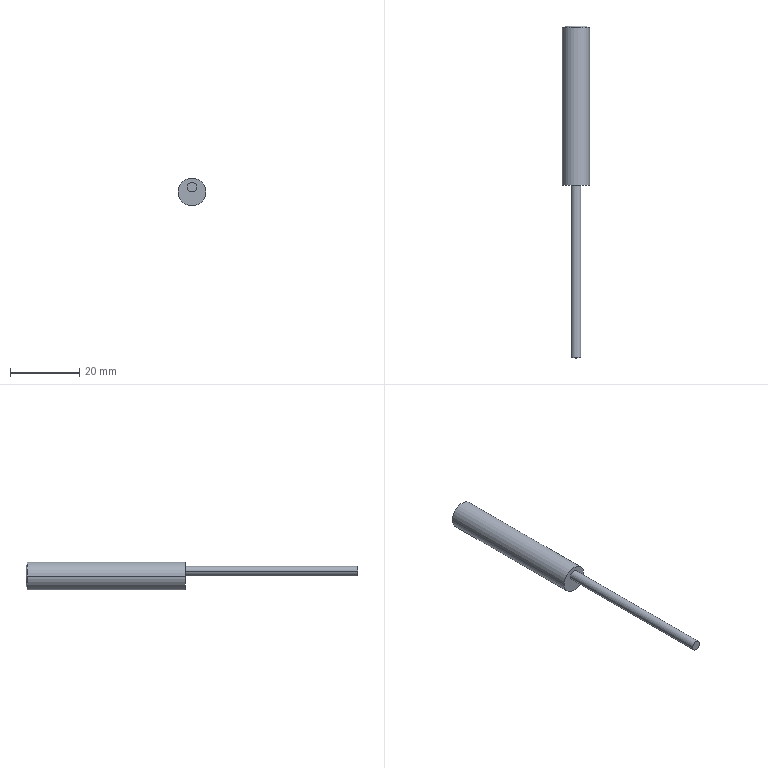Part | SolidWorks | features BaseBody 1, ICE 1, RefSurface 1 | 1 solid | 10 faces | box 8 x 96 x 8 mm | volume 2614 mm3 | cylinder 4 | plane 4 | cone 2 | commonest cylinder face diameters 2.8 x2 8 x2
STEP:
#1=CARTESIAN_POINT('',(-1.4,-46.,1.4));
#2=VERTEX_POINT('',#1);
#3=CARTESIAN_POINT('',(1.4,-46.,1.4));
#4=VERTEX_POINT('',#3);
#5=CARTESIAN_POINT('',(0.,-46.,1.4));
#6=DIRECTION('',(0.,1.,0.));
#7=DIRECTION('',(1.,0.,0.));
#8=AXIS2_PLACEMENT_3D('',#5,#6,#7);
#9=CIRCLE('',#8,1.4);
#10=EDGE_CURVE('',#2,#4,#9,.T.);
#11=ORIENTED_EDGE('',*,*,#10,.F.);
#12=CARTESIAN_POINT('',(-1.4,-96.,1.4));
#13=VERTEX_POINT('',#12);
#14=CARTESIAN_POINT('',(-1.4,-46.,1.4));
#15=DIRECTION('',(0.,-1.,0.));
#16=VECTOR('',#15,1000.);
#17=LINE('',#14,#16);
#18=EDGE_CURVE('',#2,#13,#17,.T.);
#19=ORIENTED_EDGE('',*,*,#18,.T.);
#20=CARTESIAN_POINT('',(1.4,-96.,1.4));
#21=VERTEX_POINT('',#20);
#22=CARTESIAN_POINT('',(0.,-96.,1.4));
#23=DIRECTION('',(0.,1.,0.));
#24=DIRECTION('',(1.,0.,0.));
#25=AXIS2_PLACEMENT_3D('',#22,#23,#24);
#26=CIRCLE('',#25,1.4);
#27=EDGE_CURVE('',#13,#21,#26,.T.);
#28=ORIENTED_EDGE('',*,*,#27,.T.);
#29=CARTESIAN_POINT('',(1.4,-46.,1.4));
#30=DIRECTION('',(0.,-1.,0.));
#31=VECTOR('',#30,1000.);
#32=LINE('',#29,#31);
#33=EDGE_CURVE('',#4,#21,#32,.T.);
#34=ORIENTED_EDGE('',*,*,#33,.F.);
#35=EDGE_LOOP('',(#11,#19,#28,#34));
#36=FACE_OUTER_BOUND('',#35,.T.);
#37=CARTESIAN_POINT('',(0.,-46.,1.4));
#38=DIRECTION('',(0.,-1.,0.));
#39=DIRECTION('',(1.,0.,0.));
#40=AXIS2_PLACEMENT_3D('',#37,#38,#39);
#41=CYLINDRICAL_SURFACE('',#40,1.4);
#42=ADVANCED_FACE('',(#36),#41,.T.);
#43=CARTESIAN_POINT('',(3.,0.,0.));
#44=VERTEX_POINT('',#43);
#45=CARTESIAN_POINT('',(-3.,0.,0.));
#46=VERTEX_POINT('',#45);
#47=CARTESIAN_POINT('',(0.,0.,0.));
#48=DIRECTION('',(0.,-1.,0.));
#49=DIRECTION('',(1.,0.,0.));
#50=AXIS2_PLACEMENT_3D('',#47,#48,#49);
#51=CIRCLE('',#50,3.);
#52=EDGE_CURVE('',#44,#46,#51,.T.);
#53=ORIENTED_EDGE('',*,*,#52,.T.);
#54=CARTESIAN_POINT('',(-3.3,-0.3,0.));
#55=VERTEX_POINT('',#54);
#56=CARTESIAN_POINT('',(-3.3,-0.3,0.));
#57=DIRECTION('',(-0.7071,-0.7071,0.));
#58=VECTOR('',#57,1000.);
#59=LINE('',#56,#58);
#60=EDGE_CURVE('',#46,#55,#59,.T.);
#61=ORIENTED_EDGE('',*,*,#60,.T.);
#62=CARTESIAN_POINT('',(3.3,-0.3,0.));
#63=VERTEX_POINT('',#62);
#64=CARTESIAN_POINT('',(0.,-0.3,0.));
#65=DIRECTION('',(0.,-1.,0.));
#66=DIRECTION('',(1.,0.,0.));
#67=AXIS2_PLACEMENT_3D('',#64,#65,#66);
#68=CIRCLE('',#67,3.3);
#69=EDGE_CURVE('',#63,#55,#68,.T.);
#70=ORIENTED_EDGE('',*,*,#69,.F.);
#71=CARTESIAN_POINT('',(3.3,-0.3,0.));
#72=DIRECTION('',(0.7071,-0.7071,0.));
#73=VECTOR('',#72,1000.);
#74=LINE('',#71,#73);
#75=EDGE_CURVE('',#44,#63,#74,.T.);
#76=ORIENTED_EDGE('',*,*,#75,.F.);
#77=EDGE_LOOP('',(#53,#61,#70,#76));
#78=FACE_OUTER_BOUND('',#77,.T.);
#79=CARTESIAN_POINT('',(0.,-0.3,0.));
#80=DIRECTION('',(0.,-1.,0.));
#81=DIRECTION('',(1.,0.,0.));
#82=AXIS2_PLACEMENT_3D('',#79,#80,#81);
#83=CONICAL_SURFACE('',#82,3.3,0.7854);
#84=ADVANCED_FACE('',(#78),#83,.T.);
#85=CARTESIAN_POINT('',(-4.,-46.,0.));
#86=VERTEX_POINT('',#85);
#87=CARTESIAN_POINT('',(4.,-46.,0.));
#88=VERTEX_POINT('',#87);
#89=CARTESIAN_POINT('',(0.,-46.,0.));
#90=DIRECTION('',(0.,1.,0.));
#91=DIRECTION('',(1.,0.,0.));
#92=AXIS2_PLACEMENT_3D('',#89,#90,#91);
#93=CIRCLE('',#92,4.);
#94=EDGE_CURVE('',#86,#88,#93,.T.);
#95=ORIENTED_EDGE('',*,*,#94,.T.);
#96=CARTESIAN_POINT('',(4.,-0.3,0.));
#97=VERTEX_POINT('',#96);
#98=CARTESIAN_POINT('',(4.,-57.314,0.));
#99=DIRECTION('',(0.,1.,0.));
#100=VECTOR('',#99,1000.);
#101=LINE('',#98,#100);
#102=EDGE_CURVE('',#88,#97,#101,.T.);
#103=ORIENTED_EDGE('',*,*,#102,.T.);
#104=CARTESIAN_POINT('',(-4.,-0.3,0.));
#105=VERTEX_POINT('',#104);
#106=CARTESIAN_POINT('',(0.,-0.3,0.));
#107=DIRECTION('',(0.,1.,0.));
#108=DIRECTION('',(-1.,0.,0.));
#109=AXIS2_PLACEMENT_3D('',#106,#107,#108);
#110=CIRCLE('',#109,4.);
#111=EDGE_CURVE('',#105,#97,#110,.T.);
#112=ORIENTED_EDGE('',*,*,#111,.F.);
#113=CARTESIAN_POINT('',(-4.,-57.314,0.));
#114=DIRECTION('',(0.,1.,0.));
#115=VECTOR('',#114,1000.);
#116=LINE('',#113,#115);
#117=EDGE_CURVE('',#86,#105,#116,.T.);
#118=ORIENTED_EDGE('',*,*,#117,.F.);
#119=EDGE_LOOP('',(#95,#103,#112,#118));
#120=FACE_OUTER_BOUND('',#119,.T.);
#121=CARTESIAN_POINT('',(0.,-57.314,0.));
#122=DIRECTION('',(0.,1.,0.));
#123=DIRECTION('',(-1.,0.,0.));
#124=AXIS2_PLACEMENT_3D('',#121,#122,#123);
#125=CYLINDRICAL_SURFACE('',#124,4.);
#126=ADVANCED_FACE('',(#120),#125,.T.);
#127=ORIENTED_EDGE('',*,*,#102,.F.);
#128=CARTESIAN_POINT('',(0.,-46.,0.));
#129=DIRECTION('',(0.,1.,0.));
#130=DIRECTION('',(1.,0.,0.));
#131=AXIS2_PLACEMENT_3D('',#128,#129,#130);
#132=CIRCLE('',#131,4.);
#133=EDGE_CURVE('',#88,#86,#132,.T.);
#134=ORIENTED_EDGE('',*,*,#133,.T.);
#135=ORIENTED_EDGE('',*,*,#117,.T.);
#136=CARTESIAN_POINT('',(0.,-0.3,0.));
#137=DIRECTION('',(0.,1.,0.));
#138=DIRECTION('',(-1.,0.,0.));
#139=AXIS2_PLACEMENT_3D('',#136,#137,#138);
#140=CIRCLE('',#139,4.);
#141=EDGE_CURVE('',#97,#105,#140,.T.);
#142=ORIENTED_EDGE('',*,*,#141,.F.);
#143=EDGE_LOOP('',(#127,#134,#135,#142));
#144=FACE_OUTER_BOUND('',#143,.T.);
#145=CARTESIAN_POINT('',(0.,-57.314,0.));
#146=DIRECTION('',(0.,1.,0.));
#147=DIRECTION('',(-1.,0.,0.));
#148=AXIS2_PLACEMENT_3D('',#145,#146,#147);
#149=CYLINDRICAL_SURFACE('',#148,4.);
#150=ADVANCED_FACE('',(#144),#149,.T.);
#151=ORIENTED_EDGE('',*,*,#52,.F.);
#152=CARTESIAN_POINT('',(0.,0.,0.));
#153=DIRECTION('',(0.,-1.,0.));
#154=DIRECTION('',(1.,0.,0.));
#155=AXIS2_PLACEMENT_3D('',#152,#153,#154);
#156=CIRCLE('',#155,3.);
#157=EDGE_CURVE('',#46,#44,#156,.T.);
#158=ORIENTED_EDGE('',*,*,#157,.F.);
#159=EDGE_LOOP('',(#151,#158));
#160=FACE_OUTER_BOUND('',#159,.T.);
#161=CARTESIAN_POINT('',(3.3,0.,0.));
#162=DIRECTION('',(0.,1.,0.));
#163=DIRECTION('',(-1.,0.,0.));
#164=AXIS2_PLACEMENT_3D('',#161,#162,#163);
#165=PLANE('',#164);
#166=ADVANCED_FACE('',(#160),#165,.T.);
#167=ORIENTED_EDGE('',*,*,#60,.F.);
#168=ORIENTED_EDGE('',*,*,#157,.T.);
#169=ORIENTED_EDGE('',*,*,#75,.T.);
#170=CARTESIAN_POINT('',(0.,-0.3,0.));
#171=DIRECTION('',(0.,-1.,0.));
#172=DIRECTION('',(1.,0.,0.));
#173=AXIS2_PLACEMENT_3D('',#170,#171,#172);
#174=CIRCLE('',#173,3.3);
#175=EDGE_CURVE('',#55,#63,#174,.T.);
#176=ORIENTED_EDGE('',*,*,#175,.F.);
#177=EDGE_LOOP('',(#167,#168,#169,#176));
#178=FACE_OUTER_BOUND('',#177,.T.);
#179=CARTESIAN_POINT('',(0.,-0.3,0.));
#180=DIRECTION('',(0.,-1.,0.));
#181=DIRECTION('',(1.,0.,0.));
#182=AXIS2_PLACEMENT_3D('',#179,#180,#181);
#183=CONICAL_SURFACE('',#182,3.3,0.7854);
#184=ADVANCED_FACE('',(#178),#183,.T.);
#185=ORIENTED_EDGE('',*,*,#69,.T.);
#186=ORIENTED_EDGE('',*,*,#175,.T.);
#187=EDGE_LOOP('',(#185,#186));
#188=FACE_BOUND('',#187,.T.);
#189=ORIENTED_EDGE('',*,*,#111,.T.);
#190=ORIENTED_EDGE('',*,*,#141,.T.);
#191=EDGE_LOOP('',(#189,#190));
#192=FACE_OUTER_BOUND('',#191,.T.);
#193=CARTESIAN_POINT('',(4.,-0.3,0.));
#194=DIRECTION('',(0.,1.,0.));
#195=DIRECTION('',(-1.,0.,0.));
#196=AXIS2_PLACEMENT_3D('',#193,#194,#195);
#197=PLANE('',#196);
#198=ADVANCED_FACE('',(#188,#192),#197,.T.);
#199=CARTESIAN_POINT('',(0.,-46.,1.4));
#200=DIRECTION('',(0.,1.,0.));
#201=DIRECTION('',(1.,0.,0.));
#202=AXIS2_PLACEMENT_3D('',#199,#200,#201);
#203=CIRCLE('',#202,1.4);
#204=EDGE_CURVE('',#4,#2,#203,.T.);
#205=ORIENTED_EDGE('',*,*,#204,.T.);
#206=ORIENTED_EDGE('',*,*,#10,.T.);
#207=EDGE_LOOP('',(#205,#206));
#208=FACE_BOUND('',#207,.T.);
#209=ORIENTED_EDGE('',*,*,#94,.F.);
#210=ORIENTED_EDGE('',*,*,#133,.F.);
#211=EDGE_LOOP('',(#209,#210));
#212=FACE_OUTER_BOUND('',#211,.T.);
#213=CARTESIAN_POINT('',(0.,-46.,0.));
#214=DIRECTION('',(0.,-1.,0.));
#215=DIRECTION('',(1.,0.,0.));
#216=AXIS2_PLACEMENT_3D('',#213,#214,#215);
#217=PLANE('',#216);
#218=ADVANCED_FACE('',(#208,#212),#217,.T.);
#219=ORIENTED_EDGE('',*,*,#18,.F.);
#220=ORIENTED_EDGE('',*,*,#204,.F.);
#221=ORIENTED_EDGE('',*,*,#33,.T.);
#222=CARTESIAN_POINT('',(0.,-96.,1.4));
#223=DIRECTION('',(0.,1.,0.));
#224=DIRECTION('',(1.,0.,0.));
#225=AXIS2_PLACEMENT_3D('',#222,#223,#224);
#226=CIRCLE('',#225,1.4);
#227=EDGE_CURVE('',#21,#13,#226,.T.);
#228=ORIENTED_EDGE('',*,*,#227,.T.);
#229=EDGE_LOOP('',(#219,#220,#221,#228));
#230=FACE_OUTER_BOUND('',#229,.T.);
#231=CARTESIAN_POINT('',(0.,-46.,1.4));
#232=DIRECTION('',(0.,-1.,0.));
#233=DIRECTION('',(1.,0.,0.));
#234=AXIS2_PLACEMENT_3D('',#231,#232,#233);
#235=CYLINDRICAL_SURFACE('',#234,1.4);
#236=ADVANCED_FACE('',(#230),#235,.T.);
#237=ORIENTED_EDGE('',*,*,#227,.F.);
#238=ORIENTED_EDGE('',*,*,#27,.F.);
#239=EDGE_LOOP('',(#237,#238));
#240=FACE_OUTER_BOUND('',#239,.T.);
#241=CARTESIAN_POINT('',(0.,-96.,1.4));
#242=DIRECTION('',(0.,-1.,0.));
#243=DIRECTION('',(1.,0.,0.));
#244=AXIS2_PLACEMENT_3D('',#241,#242,#243);
#245=PLANE('',#244);
#246=ADVANCED_FACE('',(#240),#245,.T.);
#247=CLOSED_SHELL('',(#42,#84,#126,#150,#166,#184,#198,#218,#236,#246));
#248=MANIFOLD_SOLID_BREP('',#247);
#249=CARTESIAN_POINT('',(0.,0.,0.));
#250=DIRECTION('',(0.,0.,1.));
#251=DIRECTION('',(1.,0.,0.));
#252=AXIS2_PLACEMENT_3D('',#249,#250,#251);
#253=(LENGTH_UNIT()NAMED_UNIT(*)SI_UNIT(.MILLI.,.METRE.));
#254=UNCERTAINTY_MEASURE_WITH_UNIT(LENGTH_MEASURE(0.00001),#253,'','');
#255=(NAMED_UNIT(*)PLANE_ANGLE_UNIT()SI_UNIT($,.RADIAN.));
#256=(NAMED_UNIT(*)SI_UNIT($,.STERADIAN.)SOLID_ANGLE_UNIT());
#257=(GEOMETRIC_REPRESENTATION_CONTEXT(3)GLOBAL_UNCERTAINTY_ASSIGNED_CONTEXT((#254))GLOBAL_UNIT_ASSIGNED_CONTEXT((#253,#255,#256))REPRESENTATION_CONTEXT('',''));
#258=ADVANCED_BREP_SHAPE_REPRESENTATION('',(#248,#252),#257);